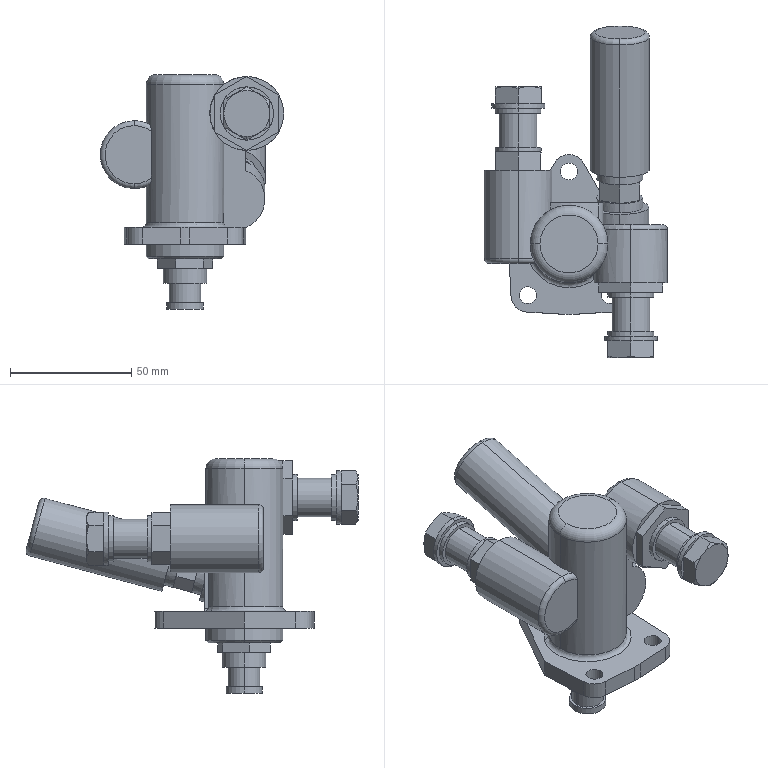Part | SolidWorks | features BaseBody 1 | 1 solid | 189 faces | box 75.75 x 136.991 x 96.8 mm | volume 170874 mm3 | plane 107 | cylinder 55 | cone 16 | torus 11 | commonest cylinder face diameters 19 x12 7 x6 32 x5 16 x4 22 x4 40 x3